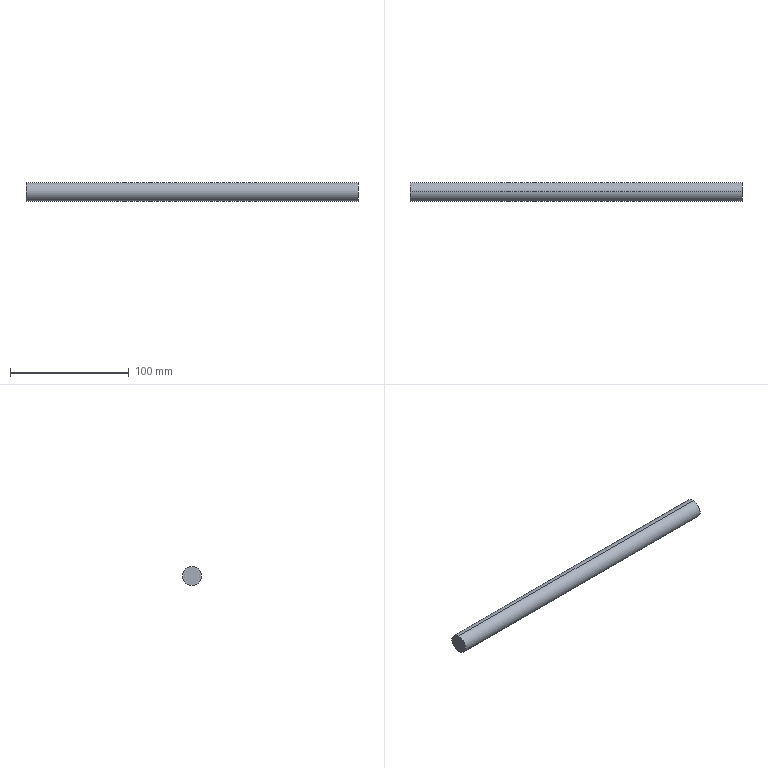Part | STEP file | A14-016 | 1 solid | 4 faces | box 280 x 16 x 16 mm | volume 56297 mm3 | cylinder 2 | plane 2 | commonest cylinder face diameters 16 x2
STEP:
#1=CARTESIAN_POINT('',(0.,0.,0.));
#2=DIRECTION('',(0.,0.,1.));
#3=DIRECTION('',(1.,0.,0.));
#4=AXIS2_PLACEMENT_3D('',#1,#2,#3);
#5=CARTESIAN_POINT('',(140.,0.,-8.));
#6=VERTEX_POINT('',#5);
#7=CARTESIAN_POINT('',(140.,0.,8.));
#8=VERTEX_POINT('',#7);
#9=CARTESIAN_POINT('',(140.,0.,0.));
#10=DIRECTION('',(1.,0.,0.));
#11=DIRECTION('',(0.,0.,-1.));
#12=AXIS2_PLACEMENT_3D('',#9,#10,#11);
#13=CIRCLE('',#12,8.);
#14=CARTESIAN_POINT('',(140.,0.,0.));
#15=DIRECTION('',(-1.,0.,0.));
#16=DIRECTION('',(0.,0.,1.));
#17=AXIS2_PLACEMENT_3D('',#14,#15,#16);
#18=CYLINDRICAL_SURFACE('',#17,8.);
#19=CARTESIAN_POINT('',(3.142,0.));
#20=DIRECTION('',(-1.,0.));
#21=VECTOR('',#20,1.);
#22=LINE('',#19,#21);
#23=(GEOMETRIC_REPRESENTATION_CONTEXT(2)PARAMETRIC_REPRESENTATION_CONTEXT()REPRESENTATION_CONTEXT('',''));
#24=DEFINITIONAL_REPRESENTATION('',(#22),#23);
#25=PCURVE('',#18,#24);
#26=CARTESIAN_POINT('',(140.,0.,0.));
#27=DIRECTION('',(1.,0.,0.));
#28=DIRECTION('',(0.,0.,-1.));
#29=AXIS2_PLACEMENT_3D('',#26,#27,#28);
#30=PLANE('',#29);
#31=CARTESIAN_POINT('',(0.,0.));
#32=DIRECTION('',(1.,0.));
#33=AXIS2_PLACEMENT_2D('',#31,#32);
#34=CIRCLE('',#33,8.);
#35=(GEOMETRIC_REPRESENTATION_CONTEXT(2)PARAMETRIC_REPRESENTATION_CONTEXT()REPRESENTATION_CONTEXT('',''));
#36=DEFINITIONAL_REPRESENTATION('',(#34),#35);
#37=PCURVE('',#30,#36);
#38=SURFACE_CURVE('',#13,(#25,#37),.PCURVE_S1.);
#39=EDGE_CURVE('',#6,#8,#38,.T.);
#40=ORIENTED_EDGE('',*,*,#39,.F.);
#41=CARTESIAN_POINT('',(-140.,0.,-8.));
#42=VERTEX_POINT('',#41);
#43=CARTESIAN_POINT('',(140.,0.,-8.));
#44=DIRECTION('',(-1.,0.,0.));
#45=VECTOR('',#44,1.);
#46=LINE('',#43,#45);
#47=CARTESIAN_POINT('',(3.142,0.));
#48=DIRECTION('',(0.,1.));
#49=VECTOR('',#48,1.);
#50=LINE('',#47,#49);
#51=(GEOMETRIC_REPRESENTATION_CONTEXT(2)PARAMETRIC_REPRESENTATION_CONTEXT()REPRESENTATION_CONTEXT('',''));
#52=DEFINITIONAL_REPRESENTATION('',(#50),#51);
#53=PCURVE('',#18,#52);
#54=CARTESIAN_POINT('',(140.,0.,0.));
#55=DIRECTION('',(-1.,0.,0.));
#56=DIRECTION('',(0.,0.,1.));
#57=AXIS2_PLACEMENT_3D('',#54,#55,#56);
#58=CYLINDRICAL_SURFACE('',#57,8.);
#59=CARTESIAN_POINT('',(3.142,0.));
#60=DIRECTION('',(0.,1.));
#61=VECTOR('',#60,1.);
#62=LINE('',#59,#61);
#63=(GEOMETRIC_REPRESENTATION_CONTEXT(2)PARAMETRIC_REPRESENTATION_CONTEXT()REPRESENTATION_CONTEXT('',''));
#64=DEFINITIONAL_REPRESENTATION('',(#62),#63);
#65=PCURVE('',#58,#64);
#66=SURFACE_CURVE('',#46,(#53,#65),.PCURVE_S1.);
#67=EDGE_CURVE('',#6,#42,#66,.T.);
#68=ORIENTED_EDGE('',*,*,#67,.T.);
#69=CARTESIAN_POINT('',(-140.,0.,8.));
#70=VERTEX_POINT('',#69);
#71=CARTESIAN_POINT('',(-140.,0.,0.));
#72=DIRECTION('',(1.,0.,0.));
#73=DIRECTION('',(0.,0.,-1.));
#74=AXIS2_PLACEMENT_3D('',#71,#72,#73);
#75=CIRCLE('',#74,8.);
#76=CARTESIAN_POINT('',(3.142,280.));
#77=DIRECTION('',(-1.,0.));
#78=VECTOR('',#77,1.);
#79=LINE('',#76,#78);
#80=(GEOMETRIC_REPRESENTATION_CONTEXT(2)PARAMETRIC_REPRESENTATION_CONTEXT()REPRESENTATION_CONTEXT('',''));
#81=DEFINITIONAL_REPRESENTATION('',(#79),#80);
#82=PCURVE('',#18,#81);
#83=CARTESIAN_POINT('',(-140.,0.,0.));
#84=DIRECTION('',(1.,0.,0.));
#85=DIRECTION('',(0.,0.,-1.));
#86=AXIS2_PLACEMENT_3D('',#83,#84,#85);
#87=PLANE('',#86);
#88=CARTESIAN_POINT('',(0.,0.));
#89=DIRECTION('',(1.,0.));
#90=AXIS2_PLACEMENT_2D('',#88,#89);
#91=CIRCLE('',#90,8.);
#92=(GEOMETRIC_REPRESENTATION_CONTEXT(2)PARAMETRIC_REPRESENTATION_CONTEXT()REPRESENTATION_CONTEXT('',''));
#93=DEFINITIONAL_REPRESENTATION('',(#91),#92);
#94=PCURVE('',#87,#93);
#95=SURFACE_CURVE('',#75,(#82,#94),.PCURVE_S1.);
#96=EDGE_CURVE('',#42,#70,#95,.T.);
#97=ORIENTED_EDGE('',*,*,#96,.T.);
#98=CARTESIAN_POINT('',(140.,0.,8.));
#99=DIRECTION('',(-1.,0.,0.));
#100=VECTOR('',#99,1.);
#101=LINE('',#98,#100);
#102=CARTESIAN_POINT('',(0.,0.));
#103=DIRECTION('',(0.,1.));
#104=VECTOR('',#103,1.);
#105=LINE('',#102,#104);
#106=(GEOMETRIC_REPRESENTATION_CONTEXT(2)PARAMETRIC_REPRESENTATION_CONTEXT()REPRESENTATION_CONTEXT('',''));
#107=DEFINITIONAL_REPRESENTATION('',(#105),#106);
#108=PCURVE('',#18,#107);
#109=CARTESIAN_POINT('',(6.283,0.));
#110=DIRECTION('',(0.,1.));
#111=VECTOR('',#110,1.);
#112=LINE('',#109,#111);
#113=(GEOMETRIC_REPRESENTATION_CONTEXT(2)PARAMETRIC_REPRESENTATION_CONTEXT()REPRESENTATION_CONTEXT('',''));
#114=DEFINITIONAL_REPRESENTATION('',(#112),#113);
#115=PCURVE('',#58,#114);
#116=SURFACE_CURVE('',#101,(#108,#115),.PCURVE_S1.);
#117=EDGE_CURVE('',#8,#70,#116,.T.);
#118=ORIENTED_EDGE('',*,*,#117,.F.);
#119=EDGE_LOOP('',(#40,#68,#97,#118));
#120=FACE_BOUND('',#119,.T.);
#121=ADVANCED_FACE('',(#120),#18,.T.);
#122=ORIENTED_EDGE('',*,*,#67,.F.);
#123=CARTESIAN_POINT('',(140.,0.,0.));
#124=DIRECTION('',(1.,0.,0.));
#125=DIRECTION('',(0.,0.,-1.));
#126=AXIS2_PLACEMENT_3D('',#123,#124,#125);
#127=CIRCLE('',#126,8.);
#128=CARTESIAN_POINT('',(9.425,0.));
#129=DIRECTION('',(-1.,0.));
#130=VECTOR('',#129,1.);
#131=LINE('',#128,#130);
#132=(GEOMETRIC_REPRESENTATION_CONTEXT(2)PARAMETRIC_REPRESENTATION_CONTEXT()REPRESENTATION_CONTEXT('',''));
#133=DEFINITIONAL_REPRESENTATION('',(#131),#132);
#134=PCURVE('',#58,#133);
#135=CARTESIAN_POINT('',(0.,0.));
#136=DIRECTION('',(1.,0.));
#137=AXIS2_PLACEMENT_2D('',#135,#136);
#138=CIRCLE('',#137,8.);
#139=(GEOMETRIC_REPRESENTATION_CONTEXT(2)PARAMETRIC_REPRESENTATION_CONTEXT()REPRESENTATION_CONTEXT('',''));
#140=DEFINITIONAL_REPRESENTATION('',(#138),#139);
#141=PCURVE('',#30,#140);
#142=SURFACE_CURVE('',#127,(#134,#141),.PCURVE_S1.);
#143=EDGE_CURVE('',#8,#6,#142,.T.);
#144=ORIENTED_EDGE('',*,*,#143,.F.);
#145=ORIENTED_EDGE('',*,*,#117,.T.);
#146=CARTESIAN_POINT('',(-140.,0.,0.));
#147=DIRECTION('',(1.,0.,0.));
#148=DIRECTION('',(0.,0.,-1.));
#149=AXIS2_PLACEMENT_3D('',#146,#147,#148);
#150=CIRCLE('',#149,8.);
#151=CARTESIAN_POINT('',(9.425,280.));
#152=DIRECTION('',(-1.,0.));
#153=VECTOR('',#152,1.);
#154=LINE('',#151,#153);
#155=(GEOMETRIC_REPRESENTATION_CONTEXT(2)PARAMETRIC_REPRESENTATION_CONTEXT()REPRESENTATION_CONTEXT('',''));
#156=DEFINITIONAL_REPRESENTATION('',(#154),#155);
#157=PCURVE('',#58,#156);
#158=CARTESIAN_POINT('',(0.,0.));
#159=DIRECTION('',(1.,0.));
#160=AXIS2_PLACEMENT_2D('',#158,#159);
#161=CIRCLE('',#160,8.);
#162=(GEOMETRIC_REPRESENTATION_CONTEXT(2)PARAMETRIC_REPRESENTATION_CONTEXT()REPRESENTATION_CONTEXT('',''));
#163=DEFINITIONAL_REPRESENTATION('',(#161),#162);
#164=PCURVE('',#87,#163);
#165=SURFACE_CURVE('',#150,(#157,#164),.PCURVE_S1.);
#166=EDGE_CURVE('',#70,#42,#165,.T.);
#167=ORIENTED_EDGE('',*,*,#166,.T.);
#168=EDGE_LOOP('',(#122,#144,#145,#167));
#169=FACE_BOUND('',#168,.T.);
#170=ADVANCED_FACE('',(#169),#58,.T.);
#171=ORIENTED_EDGE('',*,*,#143,.T.);
#172=ORIENTED_EDGE('',*,*,#39,.T.);
#173=EDGE_LOOP('',(#171,#172));
#174=FACE_BOUND('',#173,.T.);
#175=ADVANCED_FACE('',(#174),#30,.T.);
#176=ORIENTED_EDGE('',*,*,#166,.F.);
#177=ORIENTED_EDGE('',*,*,#96,.F.);
#178=EDGE_LOOP('',(#176,#177));
#179=FACE_BOUND('',#178,.T.);
#180=ADVANCED_FACE('',(#179),#87,.F.);
#181=CLOSED_SHELL('',(#121,#170,#175,#180));
#182=MANIFOLD_SOLID_BREP('',#181);
#183=(LENGTH_UNIT()NAMED_UNIT(*)SI_UNIT(.MILLI.,.METRE.));
#184=UNCERTAINTY_MEASURE_WITH_UNIT(LENGTH_MEASURE(0.0000001),#183,'','');
#185=(NAMED_UNIT(*)PLANE_ANGLE_UNIT()SI_UNIT($,.RADIAN.));
#186=(NAMED_UNIT(*)SI_UNIT($,.STERADIAN.)SOLID_ANGLE_UNIT());
#187=(GEOMETRIC_REPRESENTATION_CONTEXT(3)GLOBAL_UNCERTAINTY_ASSIGNED_CONTEXT((#184))GLOBAL_UNIT_ASSIGNED_CONTEXT((#183,#185,#186))REPRESENTATION_CONTEXT('',''));
#188=ADVANCED_BREP_SHAPE_REPRESENTATION('',(#4,#182),#187);